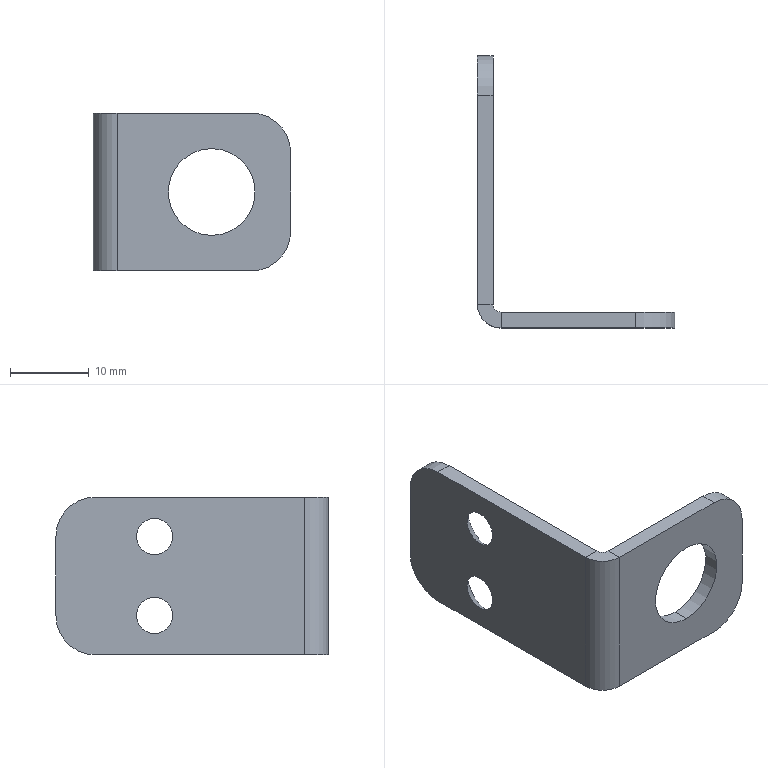Part | SolidWorks | features BreakCorner 1, FlatPattern 1, HoleWzd 1, ICE 1, SMBaseFlange 1, SheetMetal 1 | 1 solid | 24 faces | box 25 x 34.5 x 20 mm | volume 1892 mm3 | plane 12 | cylinder 8 | cone 4 | commonest cylinder face diameters 10 x4 11 x2 2 x1 6 x1
STEP:
#1=CARTESIAN_POINT('',(0.,22.,7.3));
#2=VERTEX_POINT('',#1);
#3=CARTESIAN_POINT('',(0.,22.,2.7));
#4=VERTEX_POINT('',#3);
#5=CARTESIAN_POINT('',(0.,22.,5.));
#6=DIRECTION('',(1.,0.,0.));
#7=DIRECTION('',(0.,0.,-1.));
#8=AXIS2_PLACEMENT_3D('',#5,#6,#7);
#9=CIRCLE('',#8,2.3);
#10=EDGE_CURVE('',#2,#4,#9,.T.);
#11=ORIENTED_EDGE('',*,*,#10,.F.);
#12=CARTESIAN_POINT('',(2.,22.,9.3));
#13=VERTEX_POINT('',#12);
#14=CARTESIAN_POINT('',(2.,22.,9.3));
#15=DIRECTION('',(0.7071,0.,0.7071));
#16=VECTOR('',#15,1000.);
#17=LINE('',#14,#16);
#18=EDGE_CURVE('',#2,#13,#17,.T.);
#19=ORIENTED_EDGE('',*,*,#18,.T.);
#20=CARTESIAN_POINT('',(2.,22.,0.7));
#21=VERTEX_POINT('',#20);
#22=CARTESIAN_POINT('',(2.,22.,5.));
#23=DIRECTION('',(1.,0.,0.));
#24=DIRECTION('',(0.,0.,-1.));
#25=AXIS2_PLACEMENT_3D('',#22,#23,#24);
#26=CIRCLE('',#25,4.3);
#27=EDGE_CURVE('',#13,#21,#26,.T.);
#28=ORIENTED_EDGE('',*,*,#27,.T.);
#29=CARTESIAN_POINT('',(2.,22.,0.7));
#30=DIRECTION('',(0.7071,0.,-0.7071));
#31=VECTOR('',#30,1000.);
#32=LINE('',#29,#31);
#33=EDGE_CURVE('',#4,#21,#32,.T.);
#34=ORIENTED_EDGE('',*,*,#33,.F.);
#35=EDGE_LOOP('',(#11,#19,#28,#34));
#36=FACE_OUTER_BOUND('',#35,.T.);
#37=CARTESIAN_POINT('',(2.,22.,5.));
#38=DIRECTION('',(1.,0.,0.));
#39=DIRECTION('',(0.,0.,-1.));
#40=AXIS2_PLACEMENT_3D('',#37,#38,#39);
#41=CONICAL_SURFACE('',#40,4.3,0.7854);
#42=ADVANCED_FACE('',(#36),#41,.F.);
#43=CARTESIAN_POINT('',(0.,22.,-2.7));
#44=VERTEX_POINT('',#43);
#45=CARTESIAN_POINT('',(0.,22.,-7.3));
#46=VERTEX_POINT('',#45);
#47=CARTESIAN_POINT('',(0.,22.,-5.));
#48=DIRECTION('',(1.,0.,0.));
#49=DIRECTION('',(0.,0.,-1.));
#50=AXIS2_PLACEMENT_3D('',#47,#48,#49);
#51=CIRCLE('',#50,2.3);
#52=EDGE_CURVE('',#44,#46,#51,.T.);
#53=ORIENTED_EDGE('',*,*,#52,.F.);
#54=CARTESIAN_POINT('',(2.,22.,-0.7));
#55=VERTEX_POINT('',#54);
#56=CARTESIAN_POINT('',(2.,22.,-0.7));
#57=DIRECTION('',(0.7071,0.,0.7071));
#58=VECTOR('',#57,1000.);
#59=LINE('',#56,#58);
#60=EDGE_CURVE('',#44,#55,#59,.T.);
#61=ORIENTED_EDGE('',*,*,#60,.T.);
#62=CARTESIAN_POINT('',(2.,22.,-9.3));
#63=VERTEX_POINT('',#62);
#64=CARTESIAN_POINT('',(2.,22.,-5.));
#65=DIRECTION('',(1.,0.,0.));
#66=DIRECTION('',(0.,0.,-1.));
#67=AXIS2_PLACEMENT_3D('',#64,#65,#66);
#68=CIRCLE('',#67,4.3);
#69=EDGE_CURVE('',#55,#63,#68,.T.);
#70=ORIENTED_EDGE('',*,*,#69,.T.);
#71=CARTESIAN_POINT('',(2.,22.,-9.3));
#72=DIRECTION('',(0.7071,0.,-0.7071));
#73=VECTOR('',#72,1000.);
#74=LINE('',#71,#73);
#75=EDGE_CURVE('',#46,#63,#74,.T.);
#76=ORIENTED_EDGE('',*,*,#75,.F.);
#77=EDGE_LOOP('',(#53,#61,#70,#76));
#78=FACE_OUTER_BOUND('',#77,.T.);
#79=CARTESIAN_POINT('',(2.,22.,-5.));
#80=DIRECTION('',(1.,0.,0.));
#81=DIRECTION('',(0.,0.,-1.));
#82=AXIS2_PLACEMENT_3D('',#79,#80,#81);
#83=CONICAL_SURFACE('',#82,4.3,0.7854);
#84=ADVANCED_FACE('',(#78),#83,.F.);
#85=CARTESIAN_POINT('',(15.,0.,-5.5));
#86=VERTEX_POINT('',#85);
#87=CARTESIAN_POINT('',(15.,0.,5.5));
#88=VERTEX_POINT('',#87);
#89=CARTESIAN_POINT('',(15.,0.,0.));
#90=DIRECTION('',(0.,1.,0.));
#91=DIRECTION('',(0.,0.,1.));
#92=AXIS2_PLACEMENT_3D('',#89,#90,#91);
#93=CIRCLE('',#92,5.5);
#94=EDGE_CURVE('',#86,#88,#93,.T.);
#95=ORIENTED_EDGE('',*,*,#94,.F.);
#96=CARTESIAN_POINT('',(15.,2.,-5.5));
#97=VERTEX_POINT('',#96);
#98=CARTESIAN_POINT('',(15.,0.,-5.5));
#99=DIRECTION('',(0.,1.,0.));
#100=VECTOR('',#99,1000.);
#101=LINE('',#98,#100);
#102=EDGE_CURVE('',#86,#97,#101,.T.);
#103=ORIENTED_EDGE('',*,*,#102,.T.);
#104=CARTESIAN_POINT('',(15.,2.,5.5));
#105=VERTEX_POINT('',#104);
#106=CARTESIAN_POINT('',(15.,2.,0.));
#107=DIRECTION('',(0.,1.,0.));
#108=DIRECTION('',(0.,0.,1.));
#109=AXIS2_PLACEMENT_3D('',#106,#107,#108);
#110=CIRCLE('',#109,5.5);
#111=EDGE_CURVE('',#97,#105,#110,.T.);
#112=ORIENTED_EDGE('',*,*,#111,.T.);
#113=CARTESIAN_POINT('',(15.,0.,5.5));
#114=DIRECTION('',(0.,1.,0.));
#115=VECTOR('',#114,1000.);
#116=LINE('',#113,#115);
#117=EDGE_CURVE('',#88,#105,#116,.T.);
#118=ORIENTED_EDGE('',*,*,#117,.F.);
#119=EDGE_LOOP('',(#95,#103,#112,#118));
#120=FACE_OUTER_BOUND('',#119,.T.);
#121=CARTESIAN_POINT('',(15.,0.,0.));
#122=DIRECTION('',(0.,1.,0.));
#123=DIRECTION('',(0.,0.,1.));
#124=AXIS2_PLACEMENT_3D('',#121,#122,#123);
#125=CYLINDRICAL_SURFACE('',#124,5.5);
#126=ADVANCED_FACE('',(#120),#125,.F.);
#127=CARTESIAN_POINT('',(0.,22.,5.));
#128=DIRECTION('',(1.,0.,0.));
#129=DIRECTION('',(0.,0.,-1.));
#130=AXIS2_PLACEMENT_3D('',#127,#128,#129);
#131=CIRCLE('',#130,2.3);
#132=EDGE_CURVE('',#4,#2,#131,.T.);
#133=ORIENTED_EDGE('',*,*,#132,.T.);
#134=ORIENTED_EDGE('',*,*,#10,.T.);
#135=EDGE_LOOP('',(#133,#134));
#136=FACE_BOUND('',#135,.T.);
#137=CARTESIAN_POINT('',(0.,22.,-5.));
#138=DIRECTION('',(1.,0.,0.));
#139=DIRECTION('',(0.,0.,-1.));
#140=AXIS2_PLACEMENT_3D('',#137,#138,#139);
#141=CIRCLE('',#140,2.3);
#142=EDGE_CURVE('',#46,#44,#141,.T.);
#143=ORIENTED_EDGE('',*,*,#142,.T.);
#144=ORIENTED_EDGE('',*,*,#52,.T.);
#145=EDGE_LOOP('',(#143,#144));
#146=FACE_BOUND('',#145,.T.);
#147=CARTESIAN_POINT('',(0.,29.5,10.));
#148=VERTEX_POINT('',#147);
#149=CARTESIAN_POINT('',(0.,3.,10.));
#150=VERTEX_POINT('',#149);
#151=CARTESIAN_POINT('',(0.,34.5,10.));
#152=DIRECTION('',(0.,-1.,0.));
#153=VECTOR('',#152,1000.);
#154=LINE('',#151,#153);
#155=EDGE_CURVE('',#148,#150,#154,.T.);
#156=ORIENTED_EDGE('',*,*,#155,.F.);
#157=CARTESIAN_POINT('',(0.,34.5,5.));
#158=VERTEX_POINT('',#157);
#159=CARTESIAN_POINT('',(0.,29.5,5.));
#160=DIRECTION('',(-1.,0.,0.));
#161=DIRECTION('',(0.,0.,-1.));
#162=AXIS2_PLACEMENT_3D('',#159,#160,#161);
#163=CIRCLE('',#162,5.);
#164=EDGE_CURVE('',#148,#158,#163,.T.);
#165=ORIENTED_EDGE('',*,*,#164,.T.);
#166=CARTESIAN_POINT('',(0.,34.5,-5.));
#167=VERTEX_POINT('',#166);
#168=CARTESIAN_POINT('',(0.,34.5,10.));
#169=DIRECTION('',(0.,0.,-1.));
#170=VECTOR('',#169,1000.);
#171=LINE('',#168,#170);
#172=EDGE_CURVE('',#158,#167,#171,.T.);
#173=ORIENTED_EDGE('',*,*,#172,.T.);
#174=CARTESIAN_POINT('',(0.,29.5,-10.));
#175=VERTEX_POINT('',#174);
#176=CARTESIAN_POINT('',(0.,29.5,-5.));
#177=DIRECTION('',(-1.,0.,0.));
#178=DIRECTION('',(0.,0.,-1.));
#179=AXIS2_PLACEMENT_3D('',#176,#177,#178);
#180=CIRCLE('',#179,5.);
#181=EDGE_CURVE('',#167,#175,#180,.T.);
#182=ORIENTED_EDGE('',*,*,#181,.T.);
#183=CARTESIAN_POINT('',(0.,3.,-10.));
#184=VERTEX_POINT('',#183);
#185=CARTESIAN_POINT('',(0.,34.5,-10.));
#186=DIRECTION('',(0.,-1.,0.));
#187=VECTOR('',#186,1000.);
#188=LINE('',#185,#187);
#189=EDGE_CURVE('',#175,#184,#188,.T.);
#190=ORIENTED_EDGE('',*,*,#189,.T.);
#191=CARTESIAN_POINT('',(0.,3.,10.));
#192=DIRECTION('',(0.,0.,-1.));
#193=VECTOR('',#192,1000.);
#194=LINE('',#191,#193);
#195=EDGE_CURVE('',#150,#184,#194,.T.);
#196=ORIENTED_EDGE('',*,*,#195,.F.);
#197=EDGE_LOOP('',(#156,#165,#173,#182,#190,#196));
#198=FACE_OUTER_BOUND('',#197,.T.);
#199=CARTESIAN_POINT('',(0.,34.5,10.));
#200=DIRECTION('',(1.,0.,0.));
#201=DIRECTION('',(0.,0.,-1.));
#202=AXIS2_PLACEMENT_3D('',#199,#200,#201);
#203=PLANE('',#202);
#204=ADVANCED_FACE('',(#136,#146,#198),#203,.F.);
#205=CARTESIAN_POINT('',(2.,3.,10.));
#206=VERTEX_POINT('',#205);
#207=CARTESIAN_POINT('',(0.,3.,10.));
#208=DIRECTION('',(1.,0.,0.));
#209=VECTOR('',#208,1000.);
#210=LINE('',#207,#209);
#211=EDGE_CURVE('',#150,#206,#210,.T.);
#212=ORIENTED_EDGE('',*,*,#211,.F.);
#213=CARTESIAN_POINT('',(3.,0.,10.));
#214=VERTEX_POINT('',#213);
#215=CARTESIAN_POINT('',(3.,3.,10.));
#216=DIRECTION('',(0.,0.,1.));
#217=DIRECTION('',(-1.,0.,0.));
#218=AXIS2_PLACEMENT_3D('',#215,#216,#217);
#219=CIRCLE('',#218,3.);
#220=EDGE_CURVE('',#150,#214,#219,.T.);
#221=ORIENTED_EDGE('',*,*,#220,.T.);
#222=CARTESIAN_POINT('',(3.,2.,10.));
#223=VERTEX_POINT('',#222);
#224=CARTESIAN_POINT('',(3.,2.,10.));
#225=DIRECTION('',(0.,-1.,0.));
#226=VECTOR('',#225,1000.);
#227=LINE('',#224,#226);
#228=EDGE_CURVE('',#223,#214,#227,.T.);
#229=ORIENTED_EDGE('',*,*,#228,.F.);
#230=CARTESIAN_POINT('',(3.,3.,10.));
#231=DIRECTION('',(0.,0.,1.));
#232=DIRECTION('',(1.,0.,0.));
#233=AXIS2_PLACEMENT_3D('',#230,#231,#232);
#234=CIRCLE('',#233,1.);
#235=EDGE_CURVE('',#206,#223,#234,.T.);
#236=ORIENTED_EDGE('',*,*,#235,.F.);
#237=EDGE_LOOP('',(#212,#221,#229,#236));
#238=FACE_OUTER_BOUND('',#237,.T.);
#239=CARTESIAN_POINT('',(0.,3.,10.));
#240=DIRECTION('',(0.,0.,1.));
#241=DIRECTION('',(1.,0.,0.));
#242=AXIS2_PLACEMENT_3D('',#239,#240,#241);
#243=PLANE('',#242);
#244=ADVANCED_FACE('',(#238),#243,.T.);
#245=CARTESIAN_POINT('',(2.,29.5,10.));
#246=VERTEX_POINT('',#245);
#247=CARTESIAN_POINT('',(2.,34.5,10.));
#248=DIRECTION('',(0.,-1.,0.));
#249=VECTOR('',#248,1000.);
#250=LINE('',#247,#249);
#251=EDGE_CURVE('',#246,#206,#250,.T.);
#252=ORIENTED_EDGE('',*,*,#251,.F.);
#253=CARTESIAN_POINT('',(3.,29.5,10.));
#254=DIRECTION('',(-1.,0.,0.));
#255=VECTOR('',#254,1000.);
#256=LINE('',#253,#255);
#257=EDGE_CURVE('',#246,#148,#256,.T.);
#258=ORIENTED_EDGE('',*,*,#257,.T.);
#259=ORIENTED_EDGE('',*,*,#155,.T.);
#260=ORIENTED_EDGE('',*,*,#211,.T.);
#261=EDGE_LOOP('',(#252,#258,#259,#260));
#262=FACE_OUTER_BOUND('',#261,.T.);
#263=CARTESIAN_POINT('',(3.,2.,10.));
#264=DIRECTION('',(0.,0.,1.));
#265=DIRECTION('',(1.,0.,0.));
#266=AXIS2_PLACEMENT_3D('',#263,#264,#265);
#267=PLANE('',#266);
#268=ADVANCED_FACE('',(#262),#267,.T.);
#269=CARTESIAN_POINT('',(3.,0.,-10.));
#270=VERTEX_POINT('',#269);
#271=CARTESIAN_POINT('',(3.,2.,-10.));
#272=VERTEX_POINT('',#271);
#273=CARTESIAN_POINT('',(3.,0.,-10.));
#274=DIRECTION('',(0.,1.,0.));
#275=VECTOR('',#274,1000.);
#276=LINE('',#273,#275);
#277=EDGE_CURVE('',#270,#272,#276,.T.);
#278=ORIENTED_EDGE('',*,*,#277,.F.);
#279=CARTESIAN_POINT('',(3.,3.,-10.));
#280=DIRECTION('',(0.,0.,1.));
#281=DIRECTION('',(-1.,0.,0.));
#282=AXIS2_PLACEMENT_3D('',#279,#280,#281);
#283=CIRCLE('',#282,3.);
#284=EDGE_CURVE('',#184,#270,#283,.T.);
#285=ORIENTED_EDGE('',*,*,#284,.F.);
#286=CARTESIAN_POINT('',(2.,3.,-10.));
#287=VERTEX_POINT('',#286);
#288=CARTESIAN_POINT('',(2.,3.,-10.));
#289=DIRECTION('',(-1.,0.,0.));
#290=VECTOR('',#289,1000.);
#291=LINE('',#288,#290);
#292=EDGE_CURVE('',#287,#184,#291,.T.);
#293=ORIENTED_EDGE('',*,*,#292,.F.);
#294=CARTESIAN_POINT('',(3.,3.,-10.));
#295=DIRECTION('',(0.,0.,1.));
#296=DIRECTION('',(1.,0.,0.));
#297=AXIS2_PLACEMENT_3D('',#294,#295,#296);
#298=CIRCLE('',#297,1.);
#299=EDGE_CURVE('',#287,#272,#298,.T.);
#300=ORIENTED_EDGE('',*,*,#299,.T.);
#301=EDGE_LOOP('',(#278,#285,#293,#300));
#302=FACE_OUTER_BOUND('',#301,.T.);
#303=CARTESIAN_POINT('',(3.,0.,-10.));
#304=DIRECTION('',(0.,0.,-1.));
#305=DIRECTION('',(-1.,0.,0.));
#306=AXIS2_PLACEMENT_3D('',#303,#304,#305);
#307=PLANE('',#306);
#308=ADVANCED_FACE('',(#302),#307,.T.);
#309=CARTESIAN_POINT('',(20.,2.,-10.));
#310=VERTEX_POINT('',#309);
#311=CARTESIAN_POINT('',(0.,2.,-10.));
#312=DIRECTION('',(1.,0.,0.));
#313=VECTOR('',#312,1000.);
#314=LINE('',#311,#313);
#315=EDGE_CURVE('',#272,#310,#314,.T.);
#316=ORIENTED_EDGE('',*,*,#315,.T.);
#317=CARTESIAN_POINT('',(20.,0.,-10.));
#318=VERTEX_POINT('',#317);
#319=CARTESIAN_POINT('',(20.,3.,-10.));
#320=DIRECTION('',(0.,-1.,0.));
#321=VECTOR('',#320,1000.);
#322=LINE('',#319,#321);
#323=EDGE_CURVE('',#310,#318,#322,.T.);
#324=ORIENTED_EDGE('',*,*,#323,.T.);
#325=CARTESIAN_POINT('',(0.,0.,-10.));
#326=DIRECTION('',(1.,0.,0.));
#327=VECTOR('',#326,1000.);
#328=LINE('',#325,#327);
#329=EDGE_CURVE('',#270,#318,#328,.T.);
#330=ORIENTED_EDGE('',*,*,#329,.F.);
#331=ORIENTED_EDGE('',*,*,#277,.T.);
#332=EDGE_LOOP('',(#316,#324,#330,#331));
#333=FACE_OUTER_BOUND('',#332,.T.);
#334=CARTESIAN_POINT('',(2.,3.,-10.));
#335=DIRECTION('',(0.,0.,-1.));
#336=DIRECTION('',(-1.,0.,0.));
#337=AXIS2_PLACEMENT_3D('',#334,#335,#336);
#338=PLANE('',#337);
#339=ADVANCED_FACE('',(#333),#338,.T.);
#340=CARTESIAN_POINT('',(15.,0.,0.));
#341=DIRECTION('',(0.,1.,0.));
#342=DIRECTION('',(0.,0.,1.));
#343=AXIS2_PLACEMENT_3D('',#340,#341,#342);
#344=CIRCLE('',#343,5.5);
#345=EDGE_CURVE('',#88,#86,#344,.T.);
#346=ORIENTED_EDGE('',*,*,#345,.T.);
#347=ORIENTED_EDGE('',*,*,#94,.T.);
#348=EDGE_LOOP('',(#346,#347));
#349=FACE_BOUND('',#348,.T.);
#350=CARTESIAN_POINT('',(25.,0.,5.));
#351=VERTEX_POINT('',#350);
#352=CARTESIAN_POINT('',(25.,0.,-5.));
#353=VERTEX_POINT('',#352);
#354=CARTESIAN_POINT('',(25.,0.,10.));
#355=DIRECTION('',(0.,0.,-1.));
#356=VECTOR('',#355,1000.);
#357=LINE('',#354,#356);
#358=EDGE_CURVE('',#351,#353,#357,.T.);
#359=ORIENTED_EDGE('',*,*,#358,.F.);
#360=CARTESIAN_POINT('',(20.,0.,10.));
#361=VERTEX_POINT('',#360);
#362=CARTESIAN_POINT('',(20.,0.,5.));
#363=DIRECTION('',(0.,-1.,0.));
#364=DIRECTION('',(0.,0.,1.));
#365=AXIS2_PLACEMENT_3D('',#362,#363,#364);
#366=CIRCLE('',#365,5.);
#367=EDGE_CURVE('',#351,#361,#366,.T.);
#368=ORIENTED_EDGE('',*,*,#367,.T.);
#369=CARTESIAN_POINT('',(0.,0.,10.));
#370=DIRECTION('',(1.,0.,0.));
#371=VECTOR('',#370,1000.);
#372=LINE('',#369,#371);
#373=EDGE_CURVE('',#214,#361,#372,.T.);
#374=ORIENTED_EDGE('',*,*,#373,.F.);
#375=CARTESIAN_POINT('',(3.,0.,10.));
#376=DIRECTION('',(0.,0.,-1.));
#377=VECTOR('',#376,1000.);
#378=LINE('',#375,#377);
#379=EDGE_CURVE('',#214,#270,#378,.T.);
#380=ORIENTED_EDGE('',*,*,#379,.T.);
#381=ORIENTED_EDGE('',*,*,#329,.T.);
#382=CARTESIAN_POINT('',(20.,0.,-5.));
#383=DIRECTION('',(0.,-1.,0.));
#384=DIRECTION('',(0.,0.,1.));
#385=AXIS2_PLACEMENT_3D('',#382,#383,#384);
#386=CIRCLE('',#385,5.);
#387=EDGE_CURVE('',#318,#353,#386,.T.);
#388=ORIENTED_EDGE('',*,*,#387,.T.);
#389=EDGE_LOOP('',(#359,#368,#374,#380,#381,#388));
#390=FACE_OUTER_BOUND('',#389,.T.);
#391=CARTESIAN_POINT('',(0.,0.,10.));
#392=DIRECTION('',(0.,1.,0.));
#393=DIRECTION('',(0.,0.,1.));
#394=AXIS2_PLACEMENT_3D('',#391,#392,#393);
#395=PLANE('',#394);
#396=ADVANCED_FACE('',(#349,#390),#395,.F.);
#397=CARTESIAN_POINT('',(25.,2.,5.));
#398=VERTEX_POINT('',#397);
#399=CARTESIAN_POINT('',(25.,2.,-5.));
#400=VERTEX_POINT('',#399);
#401=CARTESIAN_POINT('',(25.,2.,10.));
#402=DIRECTION('',(0.,0.,-1.));
#403=VECTOR('',#402,1000.);
#404=LINE('',#401,#403);
#405=EDGE_CURVE('',#398,#400,#404,.T.);
#406=ORIENTED_EDGE('',*,*,#405,.F.);
#407=CARTESIAN_POINT('',(25.,2.,5.));
#408=DIRECTION('',(0.,-1.,0.));
#409=VECTOR('',#408,1000.);
#410=LINE('',#407,#409);
#411=EDGE_CURVE('',#398,#351,#410,.T.);
#412=ORIENTED_EDGE('',*,*,#411,.T.);
#413=ORIENTED_EDGE('',*,*,#358,.T.);
#414=CARTESIAN_POINT('',(25.,2.,-5.));
#415=DIRECTION('',(0.,1.,0.));
#416=VECTOR('',#415,1000.);
#417=LINE('',#414,#416);
#418=EDGE_CURVE('',#353,#400,#417,.T.);
#419=ORIENTED_EDGE('',*,*,#418,.T.);
#420=EDGE_LOOP('',(#406,#412,#413,#419));
#421=FACE_OUTER_BOUND('',#420,.T.);
#422=CARTESIAN_POINT('',(25.,2.,10.));
#423=DIRECTION('',(1.,0.,0.));
#424=DIRECTION('',(0.,0.,-1.));
#425=AXIS2_PLACEMENT_3D('',#422,#423,#424);
#426=PLANE('',#425);
#427=ADVANCED_FACE('',(#421),#426,.T.);
#428=CARTESIAN_POINT('',(15.,2.,0.));
#429=DIRECTION('',(0.,1.,0.));
#430=DIRECTION('',(0.,0.,1.));
#431=AXIS2_PLACEMENT_3D('',#428,#429,#430);
#432=CIRCLE('',#431,5.5);
#433=EDGE_CURVE('',#105,#97,#432,.T.);
#434=ORIENTED_EDGE('',*,*,#433,.F.);
#435=ORIENTED_EDGE('',*,*,#111,.F.);
#436=EDGE_LOOP('',(#434,#435));
#437=FACE_BOUND('',#436,.T.);
#438=CARTESIAN_POINT('',(20.,2.,10.));
#439=VERTEX_POINT('',#438);
#440=CARTESIAN_POINT('',(0.,2.,10.));
#441=DIRECTION('',(1.,0.,0.));
#442=VECTOR('',#441,1000.);
#443=LINE('',#440,#442);
#444=EDGE_CURVE('',#223,#439,#443,.T.);
#445=ORIENTED_EDGE('',*,*,#444,.T.);
#446=CARTESIAN_POINT('',(20.,2.,5.));
#447=DIRECTION('',(0.,1.,0.));
#448=DIRECTION('',(0.,0.,1.));
#449=AXIS2_PLACEMENT_3D('',#446,#447,#448);
#450=CIRCLE('',#449,5.);
#451=EDGE_CURVE('',#439,#398,#450,.T.);
#452=ORIENTED_EDGE('',*,*,#451,.T.);
#453=ORIENTED_EDGE('',*,*,#405,.T.);
#454=CARTESIAN_POINT('',(20.,2.,-5.));
#455=DIRECTION('',(0.,1.,0.));
#456=DIRECTION('',(0.,0.,1.));
#457=AXIS2_PLACEMENT_3D('',#454,#455,#456);
#458=CIRCLE('',#457,5.);
#459=EDGE_CURVE('',#400,#310,#458,.T.);
#460=ORIENTED_EDGE('',*,*,#459,.T.);
#461=ORIENTED_EDGE('',*,*,#315,.F.);
#462=CARTESIAN_POINT('',(3.,2.,10.));
#463=DIRECTION('',(0.,0.,-1.));
#464=VECTOR('',#463,1000.);
#465=LINE('',#462,#464);
#466=EDGE_CURVE('',#223,#272,#465,.T.);
#467=ORIENTED_EDGE('',*,*,#466,.F.);
#468=EDGE_LOOP('',(#445,#452,#453,#460,#461,#467));
#469=FACE_OUTER_BOUND('',#468,.T.);
#470=CARTESIAN_POINT('',(0.,2.,10.));
#471=DIRECTION('',(0.,1.,0.));
#472=DIRECTION('',(0.,0.,1.));
#473=AXIS2_PLACEMENT_3D('',#470,#471,#472);
#474=PLANE('',#473);
#475=ADVANCED_FACE('',(#437,#469),#474,.T.);
#476=ORIENTED_EDGE('',*,*,#299,.F.);
#477=CARTESIAN_POINT('',(2.,3.,10.));
#478=DIRECTION('',(0.,0.,-1.));
#479=VECTOR('',#478,1000.);
#480=LINE('',#477,#479);
#481=EDGE_CURVE('',#206,#287,#480,.T.);
#482=ORIENTED_EDGE('',*,*,#481,.F.);
#483=ORIENTED_EDGE('',*,*,#235,.T.);
#484=ORIENTED_EDGE('',*,*,#466,.T.);
#485=EDGE_LOOP('',(#476,#482,#483,#484));
#486=FACE_OUTER_BOUND('',#485,.T.);
#487=CARTESIAN_POINT('',(3.,3.,10.));
#488=DIRECTION('',(0.,0.,-1.));
#489=DIRECTION('',(-1.,0.,0.));
#490=AXIS2_PLACEMENT_3D('',#487,#488,#489);
#491=CYLINDRICAL_SURFACE('',#490,1.);
#492=ADVANCED_FACE('',(#486),#491,.F.);
#493=CARTESIAN_POINT('',(2.,22.,5.));
#494=DIRECTION('',(1.,0.,0.));
#495=DIRECTION('',(0.,0.,-1.));
#496=AXIS2_PLACEMENT_3D('',#493,#494,#495);
#497=CIRCLE('',#496,4.3);
#498=EDGE_CURVE('',#21,#13,#497,.T.);
#499=ORIENTED_EDGE('',*,*,#498,.F.);
#500=ORIENTED_EDGE('',*,*,#27,.F.);
#501=EDGE_LOOP('',(#499,#500));
#502=FACE_BOUND('',#501,.T.);
#503=CARTESIAN_POINT('',(2.,22.,-5.));
#504=DIRECTION('',(1.,0.,0.));
#505=DIRECTION('',(0.,0.,-1.));
#506=AXIS2_PLACEMENT_3D('',#503,#504,#505);
#507=CIRCLE('',#506,4.3);
#508=EDGE_CURVE('',#63,#55,#507,.T.);
#509=ORIENTED_EDGE('',*,*,#508,.F.);
#510=ORIENTED_EDGE('',*,*,#69,.F.);
#511=EDGE_LOOP('',(#509,#510));
#512=FACE_BOUND('',#511,.T.);
#513=CARTESIAN_POINT('',(2.,34.5,5.));
#514=VERTEX_POINT('',#513);
#515=CARTESIAN_POINT('',(2.,34.5,-5.));
#516=VERTEX_POINT('',#515);
#517=CARTESIAN_POINT('',(2.,34.5,10.));
#518=DIRECTION('',(0.,0.,-1.));
#519=VECTOR('',#518,1000.);
#520=LINE('',#517,#519);
#521=EDGE_CURVE('',#514,#516,#520,.T.);
#522=ORIENTED_EDGE('',*,*,#521,.F.);
#523=CARTESIAN_POINT('',(2.,29.5,5.));
#524=DIRECTION('',(1.,0.,0.));
#525=DIRECTION('',(0.,0.,-1.));
#526=AXIS2_PLACEMENT_3D('',#523,#524,#525);
#527=CIRCLE('',#526,5.);
#528=EDGE_CURVE('',#514,#246,#527,.T.);
#529=ORIENTED_EDGE('',*,*,#528,.T.);
#530=ORIENTED_EDGE('',*,*,#251,.T.);
#531=ORIENTED_EDGE('',*,*,#481,.T.);
#532=CARTESIAN_POINT('',(2.,29.5,-10.));
#533=VERTEX_POINT('',#532);
#534=CARTESIAN_POINT('',(2.,34.5,-10.));
#535=DIRECTION('',(0.,-1.,0.));
#536=VECTOR('',#535,1000.);
#537=LINE('',#534,#536);
#538=EDGE_CURVE('',#533,#287,#537,.T.);
#539=ORIENTED_EDGE('',*,*,#538,.F.);
#540=CARTESIAN_POINT('',(2.,29.5,-5.));
#541=DIRECTION('',(1.,0.,0.));
#542=DIRECTION('',(0.,0.,-1.));
#543=AXIS2_PLACEMENT_3D('',#540,#541,#542);
#544=CIRCLE('',#543,5.);
#545=EDGE_CURVE('',#533,#516,#544,.T.);
#546=ORIENTED_EDGE('',*,*,#545,.T.);
#547=EDGE_LOOP('',(#522,#529,#530,#531,#539,#546));
#548=FACE_OUTER_BOUND('',#547,.T.);
#549=CARTESIAN_POINT('',(2.,34.5,10.));
#550=DIRECTION('',(1.,0.,0.));
#551=DIRECTION('',(0.,0.,-1.));
#552=AXIS2_PLACEMENT_3D('',#549,#550,#551);
#553=PLANE('',#552);
#554=ADVANCED_FACE('',(#502,#512,#548),#553,.T.);
#555=ORIENTED_EDGE('',*,*,#172,.F.);
#556=CARTESIAN_POINT('',(0.,34.5,5.));
#557=DIRECTION('',(1.,0.,0.));
#558=VECTOR('',#557,1000.);
#559=LINE('',#556,#558);
#560=EDGE_CURVE('',#158,#514,#559,.T.);
#561=ORIENTED_EDGE('',*,*,#560,.T.);
#562=ORIENTED_EDGE('',*,*,#521,.T.);
#563=CARTESIAN_POINT('',(0.,34.5,-5.));
#564=DIRECTION('',(-1.,0.,0.));
#565=VECTOR('',#564,1000.);
#566=LINE('',#563,#565);
#567=EDGE_CURVE('',#516,#167,#566,.T.);
#568=ORIENTED_EDGE('',*,*,#567,.T.);
#569=EDGE_LOOP('',(#555,#561,#562,#568));
#570=FACE_OUTER_BOUND('',#569,.T.);
#571=CARTESIAN_POINT('',(0.,34.5,10.));
#572=DIRECTION('',(0.,1.,0.));
#573=DIRECTION('',(0.,0.,1.));
#574=AXIS2_PLACEMENT_3D('',#571,#572,#573);
#575=PLANE('',#574);
#576=ADVANCED_FACE('',(#570),#575,.T.);
#577=ORIENTED_EDGE('',*,*,#284,.T.);
#578=ORIENTED_EDGE('',*,*,#379,.F.);
#579=ORIENTED_EDGE('',*,*,#220,.F.);
#580=ORIENTED_EDGE('',*,*,#195,.T.);
#581=EDGE_LOOP('',(#577,#578,#579,#580));
#582=FACE_OUTER_BOUND('',#581,.T.);
#583=CARTESIAN_POINT('',(3.,3.,10.));
#584=DIRECTION('',(0.,0.,-1.));
#585=DIRECTION('',(-1.,0.,0.));
#586=AXIS2_PLACEMENT_3D('',#583,#584,#585);
#587=CYLINDRICAL_SURFACE('',#586,3.);
#588=ADVANCED_FACE('',(#582),#587,.T.);
#589=ORIENTED_EDGE('',*,*,#373,.T.);
#590=CARTESIAN_POINT('',(20.,3.,10.));
#591=DIRECTION('',(0.,1.,0.));
#592=VECTOR('',#591,1000.);
#593=LINE('',#590,#592);
#594=EDGE_CURVE('',#361,#439,#593,.T.);
#595=ORIENTED_EDGE('',*,*,#594,.T.);
#596=ORIENTED_EDGE('',*,*,#444,.F.);
#597=ORIENTED_EDGE('',*,*,#228,.T.);
#598=EDGE_LOOP('',(#589,#595,#596,#597));
#599=FACE_OUTER_BOUND('',#598,.T.);
#600=CARTESIAN_POINT('',(3.,3.,10.));
#601=DIRECTION('',(0.,0.,1.));
#602=DIRECTION('',(1.,0.,0.));
#603=AXIS2_PLACEMENT_3D('',#600,#601,#602);
#604=PLANE('',#603);
#605=ADVANCED_FACE('',(#599),#604,.T.);
#606=ORIENTED_EDGE('',*,*,#189,.F.);
#607=CARTESIAN_POINT('',(2.,29.5,-10.));
#608=DIRECTION('',(1.,0.,0.));
#609=VECTOR('',#608,1000.);
#610=LINE('',#607,#609);
#611=EDGE_CURVE('',#175,#533,#610,.T.);
#612=ORIENTED_EDGE('',*,*,#611,.T.);
#613=ORIENTED_EDGE('',*,*,#538,.T.);
#614=ORIENTED_EDGE('',*,*,#292,.T.);
#615=EDGE_LOOP('',(#606,#612,#613,#614));
#616=FACE_OUTER_BOUND('',#615,.T.);
#617=CARTESIAN_POINT('',(3.,3.,-10.));
#618=DIRECTION('',(0.,0.,1.));
#619=DIRECTION('',(1.,0.,0.));
#620=AXIS2_PLACEMENT_3D('',#617,#618,#619);
#621=PLANE('',#620);
#622=ADVANCED_FACE('',(#616),#621,.F.);
#623=ORIENTED_EDGE('',*,*,#164,.F.);
#624=ORIENTED_EDGE('',*,*,#257,.F.);
#625=ORIENTED_EDGE('',*,*,#528,.F.);
#626=ORIENTED_EDGE('',*,*,#560,.F.);
#627=EDGE_LOOP('',(#623,#624,#625,#626));
#628=FACE_OUTER_BOUND('',#627,.T.);
#629=CARTESIAN_POINT('',(0.,29.5,5.));
#630=DIRECTION('',(1.,0.,0.));
#631=DIRECTION('',(0.,0.,-1.));
#632=AXIS2_PLACEMENT_3D('',#629,#630,#631);
#633=CYLINDRICAL_SURFACE('',#632,5.);
#634=ADVANCED_FACE('',(#628),#633,.T.);
#635=ORIENTED_EDGE('',*,*,#181,.F.);
#636=ORIENTED_EDGE('',*,*,#567,.F.);
#637=ORIENTED_EDGE('',*,*,#545,.F.);
#638=ORIENTED_EDGE('',*,*,#611,.F.);
#639=EDGE_LOOP('',(#635,#636,#637,#638));
#640=FACE_OUTER_BOUND('',#639,.T.);
#641=CARTESIAN_POINT('',(3.,29.5,-5.));
#642=DIRECTION('',(-1.,0.,0.));
#643=DIRECTION('',(0.,0.,1.));
#644=AXIS2_PLACEMENT_3D('',#641,#642,#643);
#645=CYLINDRICAL_SURFACE('',#644,5.);
#646=ADVANCED_FACE('',(#640),#645,.T.);
#647=ORIENTED_EDGE('',*,*,#451,.F.);
#648=ORIENTED_EDGE('',*,*,#594,.F.);
#649=ORIENTED_EDGE('',*,*,#367,.F.);
#650=ORIENTED_EDGE('',*,*,#411,.F.);
#651=EDGE_LOOP('',(#647,#648,#649,#650));
#652=FACE_OUTER_BOUND('',#651,.T.);
#653=CARTESIAN_POINT('',(20.,2.,5.));
#654=DIRECTION('',(0.,-1.,0.));
#655=DIRECTION('',(0.,0.,-1.));
#656=AXIS2_PLACEMENT_3D('',#653,#654,#655);
#657=CYLINDRICAL_SURFACE('',#656,5.);
#658=ADVANCED_FACE('',(#652),#657,.T.);
#659=ORIENTED_EDGE('',*,*,#459,.F.);
#660=ORIENTED_EDGE('',*,*,#418,.F.);
#661=ORIENTED_EDGE('',*,*,#387,.F.);
#662=ORIENTED_EDGE('',*,*,#323,.F.);
#663=EDGE_LOOP('',(#659,#660,#661,#662));
#664=FACE_OUTER_BOUND('',#663,.T.);
#665=CARTESIAN_POINT('',(20.,3.,-5.));
#666=DIRECTION('',(0.,-1.,0.));
#667=DIRECTION('',(0.,0.,-1.));
#668=AXIS2_PLACEMENT_3D('',#665,#666,#667);
#669=CYLINDRICAL_SURFACE('',#668,5.);
#670=ADVANCED_FACE('',(#664),#669,.T.);
#671=ORIENTED_EDGE('',*,*,#102,.F.);
#672=ORIENTED_EDGE('',*,*,#345,.F.);
#673=ORIENTED_EDGE('',*,*,#117,.T.);
#674=ORIENTED_EDGE('',*,*,#433,.T.);
#675=EDGE_LOOP('',(#671,#672,#673,#674));
#676=FACE_OUTER_BOUND('',#675,.T.);
#677=CARTESIAN_POINT('',(15.,0.,0.));
#678=DIRECTION('',(0.,1.,0.));
#679=DIRECTION('',(0.,0.,1.));
#680=AXIS2_PLACEMENT_3D('',#677,#678,#679);
#681=CYLINDRICAL_SURFACE('',#680,5.5);
#682=ADVANCED_FACE('',(#676),#681,.F.);
#683=ORIENTED_EDGE('',*,*,#60,.F.);
#684=ORIENTED_EDGE('',*,*,#142,.F.);
#685=ORIENTED_EDGE('',*,*,#75,.T.);
#686=ORIENTED_EDGE('',*,*,#508,.T.);
#687=EDGE_LOOP('',(#683,#684,#685,#686));
#688=FACE_OUTER_BOUND('',#687,.T.);
#689=CARTESIAN_POINT('',(2.,22.,-5.));
#690=DIRECTION('',(1.,0.,0.));
#691=DIRECTION('',(0.,0.,-1.));
#692=AXIS2_PLACEMENT_3D('',#689,#690,#691);
#693=CONICAL_SURFACE('',#692,4.3,0.7854);
#694=ADVANCED_FACE('',(#688),#693,.F.);
#695=ORIENTED_EDGE('',*,*,#18,.F.);
#696=ORIENTED_EDGE('',*,*,#132,.F.);
#697=ORIENTED_EDGE('',*,*,#33,.T.);
#698=ORIENTED_EDGE('',*,*,#498,.T.);
#699=EDGE_LOOP('',(#695,#696,#697,#698));
#700=FACE_OUTER_BOUND('',#699,.T.);
#701=CARTESIAN_POINT('',(2.,22.,5.));
#702=DIRECTION('',(1.,0.,0.));
#703=DIRECTION('',(0.,0.,-1.));
#704=AXIS2_PLACEMENT_3D('',#701,#702,#703);
#705=CONICAL_SURFACE('',#704,4.3,0.7854);
#706=ADVANCED_FACE('',(#700),#705,.F.);
#707=CLOSED_SHELL('',(#42,#84,#126,#204,#244,#268,#308,#339,#396,#427,#475,#492,#554,#576,#588,#605,#622,#634,#646,#658,#670,#682,#694,#706));
#708=MANIFOLD_SOLID_BREP('',#707);
#709=CARTESIAN_POINT('',(0.,0.,0.));
#710=DIRECTION('',(0.,0.,1.));
#711=DIRECTION('',(1.,0.,0.));
#712=AXIS2_PLACEMENT_3D('',#709,#710,#711);
#713=(LENGTH_UNIT()NAMED_UNIT(*)SI_UNIT(.MILLI.,.METRE.));
#714=UNCERTAINTY_MEASURE_WITH_UNIT(LENGTH_MEASURE(0.00001),#713,'','');
#715=(NAMED_UNIT(*)PLANE_ANGLE_UNIT()SI_UNIT($,.RADIAN.));
#716=(NAMED_UNIT(*)SI_UNIT($,.STERADIAN.)SOLID_ANGLE_UNIT());
#717=(GEOMETRIC_REPRESENTATION_CONTEXT(3)GLOBAL_UNCERTAINTY_ASSIGNED_CONTEXT((#714))GLOBAL_UNIT_ASSIGNED_CONTEXT((#713,#715,#716))REPRESENTATION_CONTEXT('',''));
#718=ADVANCED_BREP_SHAPE_REPRESENTATION('',(#708,#712),#717);